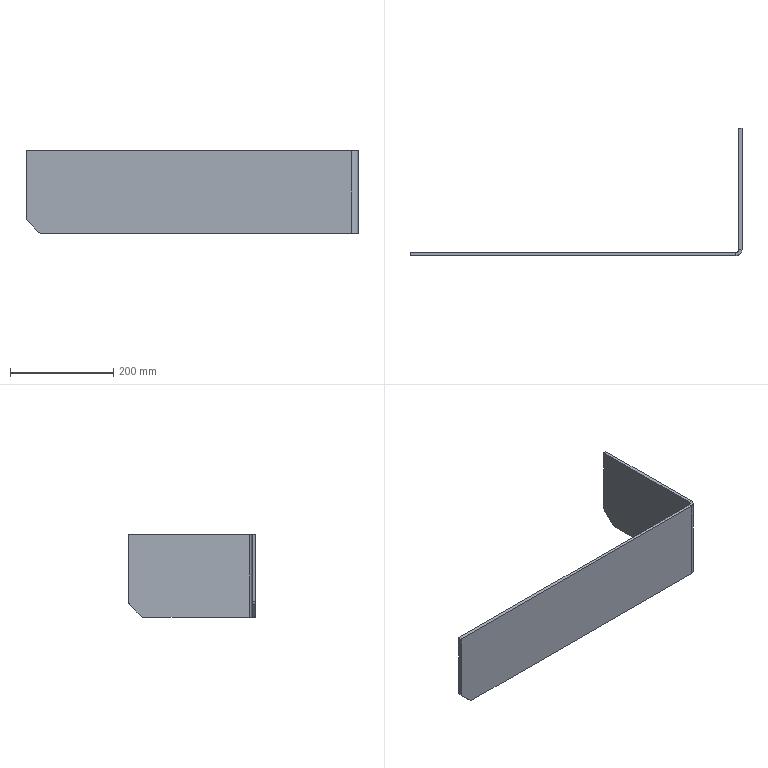Part | SolidWorks | features Chamfer 1, Fillet 1, FlatPattern 1, SMBaseFlange 1, SheetMetal 1 | 1 solid | 20 faces | box 642 x 246 x 160 mm | volume 838612 mm3 | plane 14 | cylinder 6 | commonest cylinder face diameters 14 x4 12 x1 24 x1
STEP:
#1=CARTESIAN_POINT('',(630.,0.,80.));
#2=VERTEX_POINT('',#1);
#3=CARTESIAN_POINT('',(630.,6.,80.));
#4=VERTEX_POINT('',#3);
#5=CARTESIAN_POINT('',(630.,0.,80.));
#6=DIRECTION('',(0.,1.,0.));
#7=VECTOR('',#6,1000.);
#8=LINE('',#5,#7);
#9=EDGE_CURVE('',#2,#4,#8,.T.);
#10=ORIENTED_EDGE('',*,*,#9,.F.);
#11=CARTESIAN_POINT('',(642.,12.,80.));
#12=VERTEX_POINT('',#11);
#13=CARTESIAN_POINT('',(630.,12.,80.));
#14=DIRECTION('',(0.,0.,1.));
#15=DIRECTION('',(-1.,0.,0.));
#16=AXIS2_PLACEMENT_3D('',#13,#14,#15);
#17=CIRCLE('',#16,12.);
#18=EDGE_CURVE('',#2,#12,#17,.T.);
#19=ORIENTED_EDGE('',*,*,#18,.T.);
#20=CARTESIAN_POINT('',(636.,12.,80.));
#21=VERTEX_POINT('',#20);
#22=CARTESIAN_POINT('',(636.,12.,80.));
#23=DIRECTION('',(1.,0.,0.));
#24=VECTOR('',#23,1000.);
#25=LINE('',#22,#24);
#26=EDGE_CURVE('',#21,#12,#25,.T.);
#27=ORIENTED_EDGE('',*,*,#26,.F.);
#28=CARTESIAN_POINT('',(630.,12.,80.));
#29=DIRECTION('',(0.,0.,1.));
#30=DIRECTION('',(1.,0.,0.));
#31=AXIS2_PLACEMENT_3D('',#28,#29,#30);
#32=CIRCLE('',#31,6.);
#33=EDGE_CURVE('',#4,#21,#32,.T.);
#34=ORIENTED_EDGE('',*,*,#33,.F.);
#35=EDGE_LOOP('',(#10,#19,#27,#34));
#36=FACE_OUTER_BOUND('',#35,.T.);
#37=CARTESIAN_POINT('',(630.,0.,80.));
#38=DIRECTION('',(0.,0.,1.));
#39=DIRECTION('',(1.,0.,0.));
#40=AXIS2_PLACEMENT_3D('',#37,#38,#39);
#41=PLANE('',#40);
#42=ADVANCED_FACE('',(#36),#41,.T.);
#43=CARTESIAN_POINT('',(0.,0.,80.));
#44=VERTEX_POINT('',#43);
#45=CARTESIAN_POINT('',(0.,0.,80.));
#46=DIRECTION('',(1.,0.,0.));
#47=VECTOR('',#46,1000.);
#48=LINE('',#45,#47);
#49=EDGE_CURVE('',#44,#2,#48,.T.);
#50=ORIENTED_EDGE('',*,*,#49,.T.);
#51=ORIENTED_EDGE('',*,*,#9,.T.);
#52=CARTESIAN_POINT('',(0.,6.,80.));
#53=VERTEX_POINT('',#52);
#54=CARTESIAN_POINT('',(0.,6.,80.));
#55=DIRECTION('',(1.,0.,0.));
#56=VECTOR('',#55,1000.);
#57=LINE('',#54,#56);
#58=EDGE_CURVE('',#53,#4,#57,.T.);
#59=ORIENTED_EDGE('',*,*,#58,.F.);
#60=CARTESIAN_POINT('',(0.,0.,80.));
#61=DIRECTION('',(0.,1.,0.));
#62=VECTOR('',#61,1000.);
#63=LINE('',#60,#62);
#64=EDGE_CURVE('',#44,#53,#63,.T.);
#65=ORIENTED_EDGE('',*,*,#64,.F.);
#66=EDGE_LOOP('',(#50,#51,#59,#65));
#67=FACE_OUTER_BOUND('',#66,.T.);
#68=CARTESIAN_POINT('',(636.,12.,80.));
#69=DIRECTION('',(0.,0.,1.));
#70=DIRECTION('',(1.,0.,0.));
#71=AXIS2_PLACEMENT_3D('',#68,#69,#70);
#72=PLANE('',#71);
#73=ADVANCED_FACE('',(#67),#72,.T.);
#74=CARTESIAN_POINT('',(642.,12.,-80.));
#75=VERTEX_POINT('',#74);
#76=CARTESIAN_POINT('',(636.,12.,-80.));
#77=VERTEX_POINT('',#76);
#78=CARTESIAN_POINT('',(642.,12.,-80.));
#79=DIRECTION('',(-1.,0.,0.));
#80=VECTOR('',#79,1000.);
#81=LINE('',#78,#80);
#82=EDGE_CURVE('',#75,#77,#81,.T.);
#83=ORIENTED_EDGE('',*,*,#82,.F.);
#84=CARTESIAN_POINT('',(630.,0.,-80.));
#85=VERTEX_POINT('',#84);
#86=CARTESIAN_POINT('',(630.,12.,-80.));
#87=DIRECTION('',(0.,0.,1.));
#88=DIRECTION('',(-1.,0.,0.));
#89=AXIS2_PLACEMENT_3D('',#86,#87,#88);
#90=CIRCLE('',#89,12.);
#91=EDGE_CURVE('',#85,#75,#90,.T.);
#92=ORIENTED_EDGE('',*,*,#91,.F.);
#93=CARTESIAN_POINT('',(630.,6.,-80.));
#94=VERTEX_POINT('',#93);
#95=CARTESIAN_POINT('',(630.,6.,-80.));
#96=DIRECTION('',(0.,-1.,0.));
#97=VECTOR('',#96,1000.);
#98=LINE('',#95,#97);
#99=EDGE_CURVE('',#94,#85,#98,.T.);
#100=ORIENTED_EDGE('',*,*,#99,.F.);
#101=CARTESIAN_POINT('',(630.,12.,-80.));
#102=DIRECTION('',(0.,0.,1.));
#103=DIRECTION('',(1.,0.,0.));
#104=AXIS2_PLACEMENT_3D('',#101,#102,#103);
#105=CIRCLE('',#104,6.);
#106=EDGE_CURVE('',#94,#77,#105,.T.);
#107=ORIENTED_EDGE('',*,*,#106,.T.);
#108=EDGE_LOOP('',(#83,#92,#100,#107));
#109=FACE_OUTER_BOUND('',#108,.T.);
#110=CARTESIAN_POINT('',(642.,12.,-80.));
#111=DIRECTION('',(0.,0.,-1.));
#112=DIRECTION('',(-1.,0.,0.));
#113=AXIS2_PLACEMENT_3D('',#110,#111,#112);
#114=PLANE('',#113);
#115=ADVANCED_FACE('',(#109),#114,.T.);
#116=CARTESIAN_POINT('',(636.,216.101,-80.));
#117=VERTEX_POINT('',#116);
#118=CARTESIAN_POINT('',(636.,0.,-80.));
#119=DIRECTION('',(0.,1.,0.));
#120=VECTOR('',#119,1000.);
#121=LINE('',#118,#120);
#122=EDGE_CURVE('',#77,#117,#121,.T.);
#123=ORIENTED_EDGE('',*,*,#122,.T.);
#124=CARTESIAN_POINT('',(642.,216.101,-80.));
#125=VERTEX_POINT('',#124);
#126=CARTESIAN_POINT('',(630.,216.101,-80.));
#127=DIRECTION('',(1.,0.,0.));
#128=VECTOR('',#127,1000.);
#129=LINE('',#126,#128);
#130=EDGE_CURVE('',#117,#125,#129,.T.);
#131=ORIENTED_EDGE('',*,*,#130,.T.);
#132=CARTESIAN_POINT('',(642.,0.,-80.));
#133=DIRECTION('',(0.,1.,0.));
#134=VECTOR('',#133,1000.);
#135=LINE('',#132,#134);
#136=EDGE_CURVE('',#75,#125,#135,.T.);
#137=ORIENTED_EDGE('',*,*,#136,.F.);
#138=ORIENTED_EDGE('',*,*,#82,.T.);
#139=EDGE_LOOP('',(#123,#131,#137,#138));
#140=FACE_OUTER_BOUND('',#139,.T.);
#141=CARTESIAN_POINT('',(630.,6.,-80.));
#142=DIRECTION('',(0.,0.,-1.));
#143=DIRECTION('',(-1.,0.,0.));
#144=AXIS2_PLACEMENT_3D('',#141,#142,#143);
#145=PLANE('',#144);
#146=ADVANCED_FACE('',(#140),#145,.T.);
#147=CARTESIAN_POINT('',(642.,221.05,-77.95));
#148=VERTEX_POINT('',#147);
#149=CARTESIAN_POINT('',(642.,243.95,-55.05));
#150=VERTEX_POINT('',#149);
#151=CARTESIAN_POINT('',(642.,219.,-80.));
#152=DIRECTION('',(0.,0.7071,0.7071));
#153=VECTOR('',#152,1000.);
#154=LINE('',#151,#153);
#155=EDGE_CURVE('',#148,#150,#154,.T.);
#156=ORIENTED_EDGE('',*,*,#155,.T.);
#157=CARTESIAN_POINT('',(642.,246.,-50.101));
#158=VERTEX_POINT('',#157);
#159=CARTESIAN_POINT('',(642.,239.,-50.101));
#160=DIRECTION('',(1.,0.,0.));
#161=DIRECTION('',(0.,0.,1.));
#162=AXIS2_PLACEMENT_3D('',#159,#160,#161);
#163=CIRCLE('',#162,7.);
#164=EDGE_CURVE('',#150,#158,#163,.T.);
#165=ORIENTED_EDGE('',*,*,#164,.T.);
#166=CARTESIAN_POINT('',(642.,246.,80.));
#167=VERTEX_POINT('',#166);
#168=CARTESIAN_POINT('',(642.,246.,80.));
#169=DIRECTION('',(0.,0.,-1.));
#170=VECTOR('',#169,1000.);
#171=LINE('',#168,#170);
#172=EDGE_CURVE('',#167,#158,#171,.T.);
#173=ORIENTED_EDGE('',*,*,#172,.F.);
#174=CARTESIAN_POINT('',(642.,0.,80.));
#175=DIRECTION('',(0.,1.,0.));
#176=VECTOR('',#175,1000.);
#177=LINE('',#174,#176);
#178=EDGE_CURVE('',#12,#167,#177,.T.);
#179=ORIENTED_EDGE('',*,*,#178,.F.);
#180=CARTESIAN_POINT('',(642.,12.,80.));
#181=DIRECTION('',(0.,0.,-1.));
#182=VECTOR('',#181,1000.);
#183=LINE('',#180,#182);
#184=EDGE_CURVE('',#12,#75,#183,.T.);
#185=ORIENTED_EDGE('',*,*,#184,.T.);
#186=ORIENTED_EDGE('',*,*,#136,.T.);
#187=CARTESIAN_POINT('',(642.,216.101,-73.));
#188=DIRECTION('',(1.,0.,0.));
#189=DIRECTION('',(0.,0.,1.));
#190=AXIS2_PLACEMENT_3D('',#187,#188,#189);
#191=CIRCLE('',#190,7.);
#192=EDGE_CURVE('',#125,#148,#191,.T.);
#193=ORIENTED_EDGE('',*,*,#192,.T.);
#194=EDGE_LOOP('',(#156,#165,#173,#179,#185,#186,#193));
#195=FACE_OUTER_BOUND('',#194,.T.);
#196=CARTESIAN_POINT('',(642.,0.,80.));
#197=DIRECTION('',(-1.,0.,0.));
#198=DIRECTION('',(0.,0.,1.));
#199=AXIS2_PLACEMENT_3D('',#196,#197,#198);
#200=PLANE('',#199);
#201=ADVANCED_FACE('',(#195),#200,.F.);
#202=ORIENTED_EDGE('',*,*,#172,.T.);
#203=CARTESIAN_POINT('',(636.,246.,-50.101));
#204=VERTEX_POINT('',#203);
#205=CARTESIAN_POINT('',(636.,246.,-50.101));
#206=DIRECTION('',(-1.,0.,0.));
#207=VECTOR('',#206,1000.);
#208=LINE('',#205,#207);
#209=EDGE_CURVE('',#158,#204,#208,.T.);
#210=ORIENTED_EDGE('',*,*,#209,.T.);
#211=CARTESIAN_POINT('',(636.,246.,80.));
#212=VERTEX_POINT('',#211);
#213=CARTESIAN_POINT('',(636.,246.,80.));
#214=DIRECTION('',(0.,0.,-1.));
#215=VECTOR('',#214,1000.);
#216=LINE('',#213,#215);
#217=EDGE_CURVE('',#212,#204,#216,.T.);
#218=ORIENTED_EDGE('',*,*,#217,.F.);
#219=CARTESIAN_POINT('',(636.,246.,80.));
#220=DIRECTION('',(1.,0.,0.));
#221=VECTOR('',#220,1000.);
#222=LINE('',#219,#221);
#223=EDGE_CURVE('',#212,#167,#222,.T.);
#224=ORIENTED_EDGE('',*,*,#223,.T.);
#225=EDGE_LOOP('',(#202,#210,#218,#224));
#226=FACE_OUTER_BOUND('',#225,.T.);
#227=CARTESIAN_POINT('',(636.,246.,80.));
#228=DIRECTION('',(0.,1.,0.));
#229=DIRECTION('',(0.,0.,1.));
#230=AXIS2_PLACEMENT_3D('',#227,#228,#229);
#231=PLANE('',#230);
#232=ADVANCED_FACE('',(#226),#231,.T.);
#233=ORIENTED_EDGE('',*,*,#217,.T.);
#234=CARTESIAN_POINT('',(636.,243.95,-55.05));
#235=VERTEX_POINT('',#234);
#236=CARTESIAN_POINT('',(636.,239.,-50.101));
#237=DIRECTION('',(-1.,0.,0.));
#238=DIRECTION('',(0.,0.,1.));
#239=AXIS2_PLACEMENT_3D('',#236,#237,#238);
#240=CIRCLE('',#239,7.);
#241=EDGE_CURVE('',#204,#235,#240,.T.);
#242=ORIENTED_EDGE('',*,*,#241,.T.);
#243=CARTESIAN_POINT('',(636.,221.05,-77.95));
#244=VERTEX_POINT('',#243);
#245=CARTESIAN_POINT('',(636.,189.5,-109.5));
#246=DIRECTION('',(0.,-0.7071,-0.7071));
#247=VECTOR('',#246,1000.);
#248=LINE('',#245,#247);
#249=EDGE_CURVE('',#235,#244,#248,.T.);
#250=ORIENTED_EDGE('',*,*,#249,.T.);
#251=CARTESIAN_POINT('',(636.,216.101,-73.));
#252=DIRECTION('',(-1.,0.,0.));
#253=DIRECTION('',(0.,0.,1.));
#254=AXIS2_PLACEMENT_3D('',#251,#252,#253);
#255=CIRCLE('',#254,7.);
#256=EDGE_CURVE('',#244,#117,#255,.T.);
#257=ORIENTED_EDGE('',*,*,#256,.T.);
#258=ORIENTED_EDGE('',*,*,#122,.F.);
#259=CARTESIAN_POINT('',(636.,12.,80.));
#260=DIRECTION('',(0.,0.,-1.));
#261=VECTOR('',#260,1000.);
#262=LINE('',#259,#261);
#263=EDGE_CURVE('',#21,#77,#262,.T.);
#264=ORIENTED_EDGE('',*,*,#263,.F.);
#265=CARTESIAN_POINT('',(636.,0.,80.));
#266=DIRECTION('',(0.,1.,0.));
#267=VECTOR('',#266,1000.);
#268=LINE('',#265,#267);
#269=EDGE_CURVE('',#21,#212,#268,.T.);
#270=ORIENTED_EDGE('',*,*,#269,.T.);
#271=EDGE_LOOP('',(#233,#242,#250,#257,#258,#264,#270));
#272=FACE_OUTER_BOUND('',#271,.T.);
#273=CARTESIAN_POINT('',(636.,0.,80.));
#274=DIRECTION('',(-1.,0.,0.));
#275=DIRECTION('',(0.,0.,1.));
#276=AXIS2_PLACEMENT_3D('',#273,#274,#275);
#277=PLANE('',#276);
#278=ADVANCED_FACE('',(#272),#277,.T.);
#279=ORIENTED_EDGE('',*,*,#106,.F.);
#280=CARTESIAN_POINT('',(630.,6.,80.));
#281=DIRECTION('',(0.,0.,-1.));
#282=VECTOR('',#281,1000.);
#283=LINE('',#280,#282);
#284=EDGE_CURVE('',#4,#94,#283,.T.);
#285=ORIENTED_EDGE('',*,*,#284,.F.);
#286=ORIENTED_EDGE('',*,*,#33,.T.);
#287=ORIENTED_EDGE('',*,*,#263,.T.);
#288=EDGE_LOOP('',(#279,#285,#286,#287));
#289=FACE_OUTER_BOUND('',#288,.T.);
#290=CARTESIAN_POINT('',(630.,12.,80.));
#291=DIRECTION('',(0.,0.,-1.));
#292=DIRECTION('',(-1.,0.,0.));
#293=AXIS2_PLACEMENT_3D('',#290,#291,#292);
#294=CYLINDRICAL_SURFACE('',#293,6.);
#295=ADVANCED_FACE('',(#289),#294,.F.);
#296=CARTESIAN_POINT('',(24.95,6.,-77.95));
#297=VERTEX_POINT('',#296);
#298=CARTESIAN_POINT('',(2.05,6.,-55.05));
#299=VERTEX_POINT('',#298);
#300=CARTESIAN_POINT('',(-66.5,6.,13.5));
#301=DIRECTION('',(-0.7071,0.,0.7071));
#302=VECTOR('',#301,1000.);
#303=LINE('',#300,#302);
#304=EDGE_CURVE('',#297,#299,#303,.T.);
#305=ORIENTED_EDGE('',*,*,#304,.T.);
#306=CARTESIAN_POINT('',(0.,6.,-50.101));
#307=VERTEX_POINT('',#306);
#308=CARTESIAN_POINT('',(7.,6.,-50.101));
#309=DIRECTION('',(0.,1.,0.));
#310=DIRECTION('',(0.,0.,1.));
#311=AXIS2_PLACEMENT_3D('',#308,#309,#310);
#312=CIRCLE('',#311,7.);
#313=EDGE_CURVE('',#299,#307,#312,.T.);
#314=ORIENTED_EDGE('',*,*,#313,.T.);
#315=CARTESIAN_POINT('',(0.,6.,80.));
#316=DIRECTION('',(0.,0.,-1.));
#317=VECTOR('',#316,1000.);
#318=LINE('',#315,#317);
#319=EDGE_CURVE('',#53,#307,#318,.T.);
#320=ORIENTED_EDGE('',*,*,#319,.F.);
#321=ORIENTED_EDGE('',*,*,#58,.T.);
#322=ORIENTED_EDGE('',*,*,#284,.T.);
#323=CARTESIAN_POINT('',(29.899,6.,-80.));
#324=VERTEX_POINT('',#323);
#325=CARTESIAN_POINT('',(0.,6.,-80.));
#326=DIRECTION('',(1.,0.,0.));
#327=VECTOR('',#326,1000.);
#328=LINE('',#325,#327);
#329=EDGE_CURVE('',#324,#94,#328,.T.);
#330=ORIENTED_EDGE('',*,*,#329,.F.);
#331=CARTESIAN_POINT('',(29.899,6.,-73.));
#332=DIRECTION('',(0.,1.,0.));
#333=DIRECTION('',(0.,0.,1.));
#334=AXIS2_PLACEMENT_3D('',#331,#332,#333);
#335=CIRCLE('',#334,7.);
#336=EDGE_CURVE('',#324,#297,#335,.T.);
#337=ORIENTED_EDGE('',*,*,#336,.T.);
#338=EDGE_LOOP('',(#305,#314,#320,#321,#322,#330,#337));
#339=FACE_OUTER_BOUND('',#338,.T.);
#340=CARTESIAN_POINT('',(0.,6.,80.));
#341=DIRECTION('',(0.,1.,0.));
#342=DIRECTION('',(0.,0.,1.));
#343=AXIS2_PLACEMENT_3D('',#340,#341,#342);
#344=PLANE('',#343);
#345=ADVANCED_FACE('',(#339),#344,.T.);
#346=ORIENTED_EDGE('',*,*,#319,.T.);
#347=CARTESIAN_POINT('',(0.,0.,-50.101));
#348=VERTEX_POINT('',#347);
#349=CARTESIAN_POINT('',(0.,0.,-50.101));
#350=DIRECTION('',(0.,-1.,0.));
#351=VECTOR('',#350,1000.);
#352=LINE('',#349,#351);
#353=EDGE_CURVE('',#307,#348,#352,.T.);
#354=ORIENTED_EDGE('',*,*,#353,.T.);
#355=CARTESIAN_POINT('',(0.,0.,80.));
#356=DIRECTION('',(0.,0.,-1.));
#357=VECTOR('',#356,1000.);
#358=LINE('',#355,#357);
#359=EDGE_CURVE('',#44,#348,#358,.T.);
#360=ORIENTED_EDGE('',*,*,#359,.F.);
#361=ORIENTED_EDGE('',*,*,#64,.T.);
#362=EDGE_LOOP('',(#346,#354,#360,#361));
#363=FACE_OUTER_BOUND('',#362,.T.);
#364=CARTESIAN_POINT('',(0.,0.,80.));
#365=DIRECTION('',(-1.,0.,0.));
#366=DIRECTION('',(0.,0.,1.));
#367=AXIS2_PLACEMENT_3D('',#364,#365,#366);
#368=PLANE('',#367);
#369=ADVANCED_FACE('',(#363),#368,.T.);
#370=ORIENTED_EDGE('',*,*,#359,.T.);
#371=CARTESIAN_POINT('',(2.05,0.,-55.05));
#372=VERTEX_POINT('',#371);
#373=CARTESIAN_POINT('',(7.,0.,-50.101));
#374=DIRECTION('',(0.,-1.,0.));
#375=DIRECTION('',(0.,0.,1.));
#376=AXIS2_PLACEMENT_3D('',#373,#374,#375);
#377=CIRCLE('',#376,7.);
#378=EDGE_CURVE('',#348,#372,#377,.T.);
#379=ORIENTED_EDGE('',*,*,#378,.T.);
#380=CARTESIAN_POINT('',(24.95,0.,-77.95));
#381=VERTEX_POINT('',#380);
#382=CARTESIAN_POINT('',(27.,0.,-80.));
#383=DIRECTION('',(0.7071,0.,-0.7071));
#384=VECTOR('',#383,1000.);
#385=LINE('',#382,#384);
#386=EDGE_CURVE('',#372,#381,#385,.T.);
#387=ORIENTED_EDGE('',*,*,#386,.T.);
#388=CARTESIAN_POINT('',(29.899,0.,-80.));
#389=VERTEX_POINT('',#388);
#390=CARTESIAN_POINT('',(29.899,0.,-73.));
#391=DIRECTION('',(0.,-1.,0.));
#392=DIRECTION('',(0.,0.,1.));
#393=AXIS2_PLACEMENT_3D('',#390,#391,#392);
#394=CIRCLE('',#393,7.);
#395=EDGE_CURVE('',#381,#389,#394,.T.);
#396=ORIENTED_EDGE('',*,*,#395,.T.);
#397=CARTESIAN_POINT('',(0.,0.,-80.));
#398=DIRECTION('',(1.,0.,0.));
#399=VECTOR('',#398,1000.);
#400=LINE('',#397,#399);
#401=EDGE_CURVE('',#389,#85,#400,.T.);
#402=ORIENTED_EDGE('',*,*,#401,.T.);
#403=CARTESIAN_POINT('',(630.,0.,80.));
#404=DIRECTION('',(0.,0.,-1.));
#405=VECTOR('',#404,1000.);
#406=LINE('',#403,#405);
#407=EDGE_CURVE('',#2,#85,#406,.T.);
#408=ORIENTED_EDGE('',*,*,#407,.F.);
#409=ORIENTED_EDGE('',*,*,#49,.F.);
#410=EDGE_LOOP('',(#370,#379,#387,#396,#402,#408,#409));
#411=FACE_OUTER_BOUND('',#410,.T.);
#412=CARTESIAN_POINT('',(0.,0.,80.));
#413=DIRECTION('',(0.,1.,0.));
#414=DIRECTION('',(0.,0.,1.));
#415=AXIS2_PLACEMENT_3D('',#412,#413,#414);
#416=PLANE('',#415);
#417=ADVANCED_FACE('',(#411),#416,.F.);
#418=ORIENTED_EDGE('',*,*,#91,.T.);
#419=ORIENTED_EDGE('',*,*,#184,.F.);
#420=ORIENTED_EDGE('',*,*,#18,.F.);
#421=ORIENTED_EDGE('',*,*,#407,.T.);
#422=EDGE_LOOP('',(#418,#419,#420,#421));
#423=FACE_OUTER_BOUND('',#422,.T.);
#424=CARTESIAN_POINT('',(630.,12.,80.));
#425=DIRECTION('',(0.,0.,-1.));
#426=DIRECTION('',(-1.,0.,0.));
#427=AXIS2_PLACEMENT_3D('',#424,#425,#426);
#428=CYLINDRICAL_SURFACE('',#427,12.);
#429=ADVANCED_FACE('',(#423),#428,.T.);
#430=ORIENTED_EDGE('',*,*,#178,.T.);
#431=ORIENTED_EDGE('',*,*,#223,.F.);
#432=ORIENTED_EDGE('',*,*,#269,.F.);
#433=ORIENTED_EDGE('',*,*,#26,.T.);
#434=EDGE_LOOP('',(#430,#431,#432,#433));
#435=FACE_OUTER_BOUND('',#434,.T.);
#436=CARTESIAN_POINT('',(630.,12.,80.));
#437=DIRECTION('',(0.,0.,1.));
#438=DIRECTION('',(1.,0.,0.));
#439=AXIS2_PLACEMENT_3D('',#436,#437,#438);
#440=PLANE('',#439);
#441=ADVANCED_FACE('',(#435),#440,.T.);
#442=ORIENTED_EDGE('',*,*,#401,.F.);
#443=CARTESIAN_POINT('',(29.899,6.,-80.));
#444=DIRECTION('',(0.,1.,0.));
#445=VECTOR('',#444,1000.);
#446=LINE('',#443,#445);
#447=EDGE_CURVE('',#389,#324,#446,.T.);
#448=ORIENTED_EDGE('',*,*,#447,.T.);
#449=ORIENTED_EDGE('',*,*,#329,.T.);
#450=ORIENTED_EDGE('',*,*,#99,.T.);
#451=EDGE_LOOP('',(#442,#448,#449,#450));
#452=FACE_OUTER_BOUND('',#451,.T.);
#453=CARTESIAN_POINT('',(630.,12.,-80.));
#454=DIRECTION('',(0.,0.,1.));
#455=DIRECTION('',(1.,0.,0.));
#456=AXIS2_PLACEMENT_3D('',#453,#454,#455);
#457=PLANE('',#456);
#458=ADVANCED_FACE('',(#452),#457,.F.);
#459=ORIENTED_EDGE('',*,*,#249,.F.);
#460=CARTESIAN_POINT('',(630.,243.95,-55.05));
#461=DIRECTION('',(1.,0.,0.));
#462=VECTOR('',#461,1000.);
#463=LINE('',#460,#462);
#464=EDGE_CURVE('',#235,#150,#463,.T.);
#465=ORIENTED_EDGE('',*,*,#464,.T.);
#466=ORIENTED_EDGE('',*,*,#155,.F.);
#467=CARTESIAN_POINT('',(630.,221.05,-77.95));
#468=DIRECTION('',(-1.,0.,0.));
#469=VECTOR('',#468,1000.);
#470=LINE('',#467,#469);
#471=EDGE_CURVE('',#148,#244,#470,.T.);
#472=ORIENTED_EDGE('',*,*,#471,.T.);
#473=EDGE_LOOP('',(#459,#465,#466,#472));
#474=FACE_OUTER_BOUND('',#473,.T.);
#475=CARTESIAN_POINT('',(630.,219.,-80.));
#476=DIRECTION('',(0.,-0.7071,0.7071));
#477=DIRECTION('',(1.,0.,0.));
#478=AXIS2_PLACEMENT_3D('',#475,#476,#477);
#479=PLANE('',#478);
#480=ADVANCED_FACE('',(#474),#479,.F.);
#481=ORIENTED_EDGE('',*,*,#386,.F.);
#482=CARTESIAN_POINT('',(2.05,12.,-55.05));
#483=DIRECTION('',(0.,1.,0.));
#484=VECTOR('',#483,1000.);
#485=LINE('',#482,#484);
#486=EDGE_CURVE('',#372,#299,#485,.T.);
#487=ORIENTED_EDGE('',*,*,#486,.T.);
#488=ORIENTED_EDGE('',*,*,#304,.F.);
#489=CARTESIAN_POINT('',(24.95,0.,-77.95));
#490=DIRECTION('',(0.,-1.,0.));
#491=VECTOR('',#490,1000.);
#492=LINE('',#489,#491);
#493=EDGE_CURVE('',#297,#381,#492,.T.);
#494=ORIENTED_EDGE('',*,*,#493,.T.);
#495=EDGE_LOOP('',(#481,#487,#488,#494));
#496=FACE_OUTER_BOUND('',#495,.T.);
#497=CARTESIAN_POINT('',(27.,12.,-80.));
#498=DIRECTION('',(-0.7071,0.,-0.7071));
#499=DIRECTION('',(0.,-1.,0.));
#500=AXIS2_PLACEMENT_3D('',#497,#498,#499);
#501=PLANE('',#500);
#502=ADVANCED_FACE('',(#496),#501,.T.);
#503=ORIENTED_EDGE('',*,*,#313,.F.);
#504=ORIENTED_EDGE('',*,*,#486,.F.);
#505=ORIENTED_EDGE('',*,*,#378,.F.);
#506=ORIENTED_EDGE('',*,*,#353,.F.);
#507=EDGE_LOOP('',(#503,#504,#505,#506));
#508=FACE_OUTER_BOUND('',#507,.T.);
#509=CARTESIAN_POINT('',(7.,0.,-50.101));
#510=DIRECTION('',(0.,-1.,0.));
#511=DIRECTION('',(0.,0.,-1.));
#512=AXIS2_PLACEMENT_3D('',#509,#510,#511);
#513=CYLINDRICAL_SURFACE('',#512,7.);
#514=ADVANCED_FACE('',(#508),#513,.T.);
#515=ORIENTED_EDGE('',*,*,#395,.F.);
#516=ORIENTED_EDGE('',*,*,#493,.F.);
#517=ORIENTED_EDGE('',*,*,#336,.F.);
#518=ORIENTED_EDGE('',*,*,#447,.F.);
#519=EDGE_LOOP('',(#515,#516,#517,#518));
#520=FACE_OUTER_BOUND('',#519,.T.);
#521=CARTESIAN_POINT('',(29.899,12.,-73.));
#522=DIRECTION('',(0.,-1.,0.));
#523=DIRECTION('',(0.,0.,-1.));
#524=AXIS2_PLACEMENT_3D('',#521,#522,#523);
#525=CYLINDRICAL_SURFACE('',#524,7.);
#526=ADVANCED_FACE('',(#520),#525,.T.);
#527=ORIENTED_EDGE('',*,*,#164,.F.);
#528=ORIENTED_EDGE('',*,*,#464,.F.);
#529=ORIENTED_EDGE('',*,*,#241,.F.);
#530=ORIENTED_EDGE('',*,*,#209,.F.);
#531=EDGE_LOOP('',(#527,#528,#529,#530));
#532=FACE_OUTER_BOUND('',#531,.T.);
#533=CARTESIAN_POINT('',(636.,239.,-50.101));
#534=DIRECTION('',(1.,0.,0.));
#535=DIRECTION('',(0.,0.,-1.));
#536=AXIS2_PLACEMENT_3D('',#533,#534,#535);
#537=CYLINDRICAL_SURFACE('',#536,7.);
#538=ADVANCED_FACE('',(#532),#537,.T.);
#539=ORIENTED_EDGE('',*,*,#256,.F.);
#540=ORIENTED_EDGE('',*,*,#471,.F.);
#541=ORIENTED_EDGE('',*,*,#192,.F.);
#542=ORIENTED_EDGE('',*,*,#130,.F.);
#543=EDGE_LOOP('',(#539,#540,#541,#542));
#544=FACE_OUTER_BOUND('',#543,.T.);
#545=CARTESIAN_POINT('',(630.,216.101,-73.));
#546=DIRECTION('',(-1.,0.,0.));
#547=DIRECTION('',(0.,0.,1.));
#548=AXIS2_PLACEMENT_3D('',#545,#546,#547);
#549=CYLINDRICAL_SURFACE('',#548,7.);
#550=ADVANCED_FACE('',(#544),#549,.T.);
#551=CLOSED_SHELL('',(#42,#73,#115,#146,#201,#232,#278,#295,#345,#369,#417,#429,#441,#458,#480,#502,#514,#526,#538,#550));
#552=MANIFOLD_SOLID_BREP('',#551);
#553=CARTESIAN_POINT('',(0.,0.,0.));
#554=DIRECTION('',(0.,0.,1.));
#555=DIRECTION('',(1.,0.,0.));
#556=AXIS2_PLACEMENT_3D('',#553,#554,#555);
#557=(LENGTH_UNIT()NAMED_UNIT(*)SI_UNIT(.MILLI.,.METRE.));
#558=UNCERTAINTY_MEASURE_WITH_UNIT(LENGTH_MEASURE(0.00001),#557,'','');
#559=(NAMED_UNIT(*)PLANE_ANGLE_UNIT()SI_UNIT($,.RADIAN.));
#560=(NAMED_UNIT(*)SI_UNIT($,.STERADIAN.)SOLID_ANGLE_UNIT());
#561=(GEOMETRIC_REPRESENTATION_CONTEXT(3)GLOBAL_UNCERTAINTY_ASSIGNED_CONTEXT((#558))GLOBAL_UNIT_ASSIGNED_CONTEXT((#557,#559,#560))REPRESENTATION_CONTEXT('',''));
#562=ADVANCED_BREP_SHAPE_REPRESENTATION('',(#552,#556),#561);